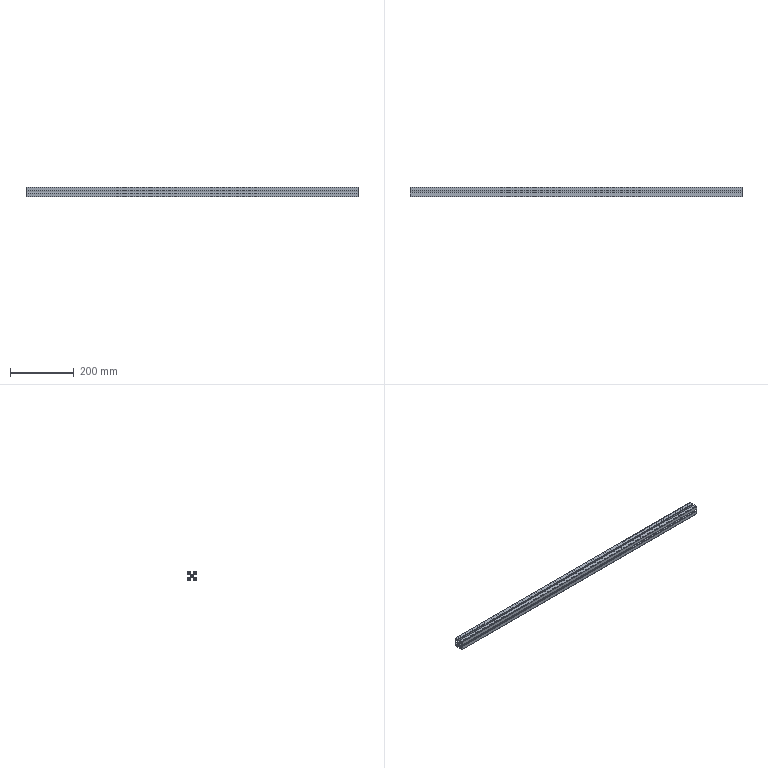Part | SolidWorks | features WeldMemberFeat 1, WeldmentFeature 1 | 1 solid | 64 faces | box 1040 x 30 x 30 mm | volume 414964 mm3 | plane 42 | cylinder 22 | commonest cylinder face diameters 6 x8 15.262 x8 2 x4 5 x2